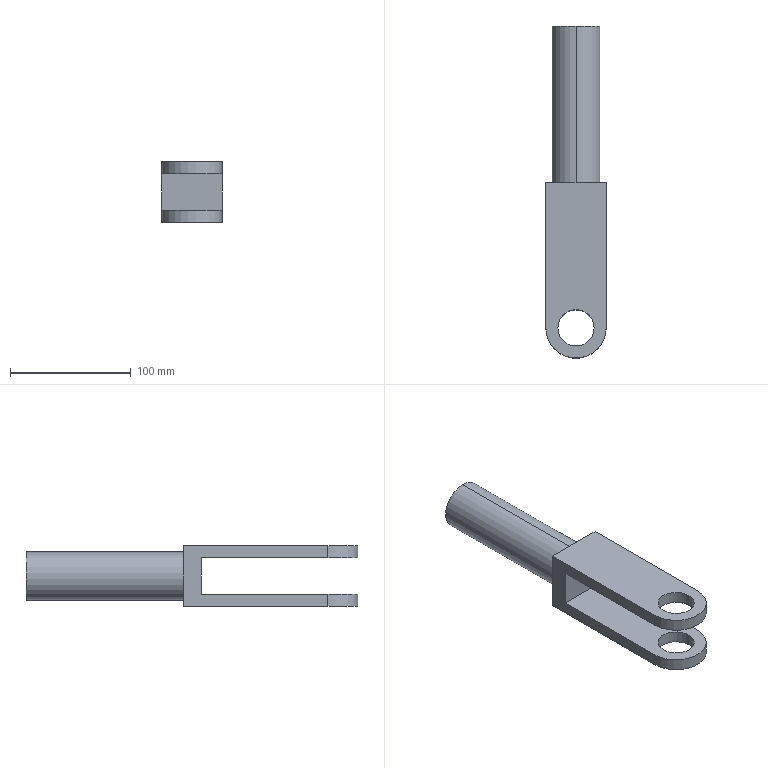Part | SolidWorks | features ICE 4, Extrusion 1, Helix 1, SweepCut 1 | 1 solid | 48 faces | box 50 x 275 x 50 mm | volume 242465 mm3 | cylinder 33 | plane 11 | spline 4 | commonest cylinder face diameters 25 x25 30 x4 40 x2 50 x2